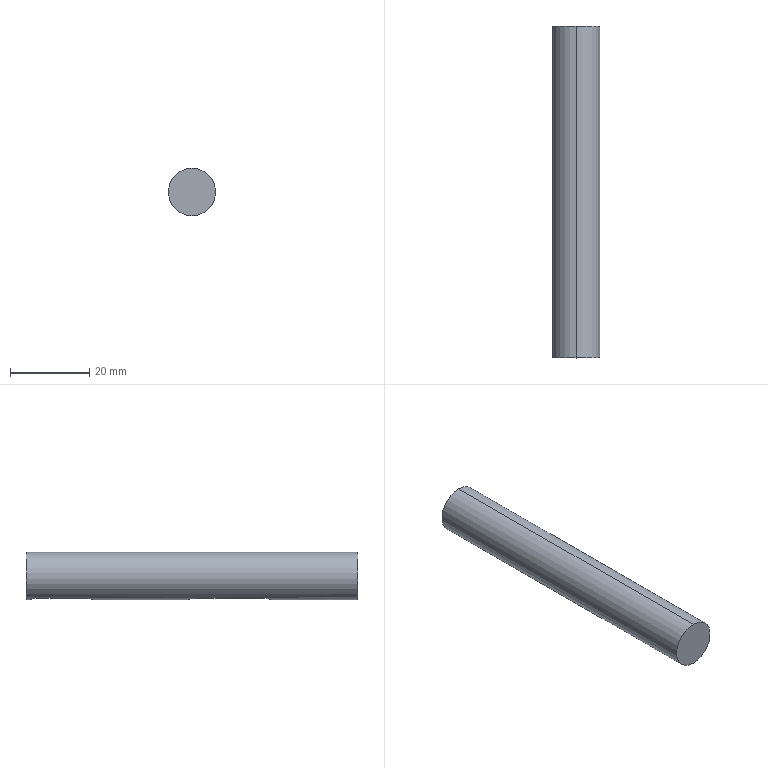Part | 1 solid | 14 faces | box 12 x 84 x 12 mm | volume 9233 mm3 | plane 8 | cylinder 6 | commonest cylinder face diameters 4 x4 12 x2
STEP:
#1=CARTESIAN_POINT('',(0.,84.,6.));
#2=VERTEX_POINT('',#1);
#3=CARTESIAN_POINT('',(0.,84.,-6.));
#4=VERTEX_POINT('',#3);
#5=CARTESIAN_POINT('',(0.,84.,0.));
#6=DIRECTION('',(0.,1.,0.));
#7=DIRECTION('',(0.,0.,1.));
#8=AXIS2_PLACEMENT_3D('',#5,#6,#7);
#9=CIRCLE('',#8,6.);
#10=EDGE_CURVE('',#2,#4,#9,.T.);
#11=ORIENTED_EDGE('',*,*,#10,.F.);
#12=CARTESIAN_POINT('',(0.,0.,6.));
#13=VERTEX_POINT('',#12);
#14=CARTESIAN_POINT('',(0.,84.,6.));
#15=DIRECTION('',(0.,-1.,0.));
#16=VECTOR('',#15,1000.);
#17=LINE('',#14,#16);
#18=EDGE_CURVE('',#2,#13,#17,.T.);
#19=ORIENTED_EDGE('',*,*,#18,.T.);
#20=CARTESIAN_POINT('',(0.,0.,-6.));
#21=VERTEX_POINT('',#20);
#22=CARTESIAN_POINT('',(0.,0.,0.));
#23=DIRECTION('',(0.,1.,0.));
#24=DIRECTION('',(0.,0.,1.));
#25=AXIS2_PLACEMENT_3D('',#22,#23,#24);
#26=CIRCLE('',#25,6.);
#27=EDGE_CURVE('',#13,#21,#26,.T.);
#28=ORIENTED_EDGE('',*,*,#27,.T.);
#29=CARTESIAN_POINT('',(0.,22.,-6.));
#30=VERTEX_POINT('',#29);
#31=CARTESIAN_POINT('',(0.,84.,-6.));
#32=DIRECTION('',(0.,-1.,0.));
#33=VECTOR('',#32,1000.);
#34=LINE('',#31,#33);
#35=EDGE_CURVE('',#30,#21,#34,.T.);
#36=ORIENTED_EDGE('',*,*,#35,.F.);
#37=CARTESIAN_POINT('',(2.,24.,-5.657));
#38=VERTEX_POINT('',#37);
#39=CARTESIAN_POINT('',(0.,22.,-6.));
#40=CARTESIAN_POINT('',(0.1314,22.,-6.));
#41=CARTESIAN_POINT('',(0.2649,22.013,-5.996));
#42=CARTESIAN_POINT('',(0.5219,22.065,-5.979));
#43=CARTESIAN_POINT('',(0.647,22.103,-5.966));
#44=CARTESIAN_POINT('',(0.8902,22.204,-5.935));
#45=CARTESIAN_POINT('',(1.006,22.266,-5.916));
#46=CARTESIAN_POINT('',(1.221,22.411,-5.875));
#47=CARTESIAN_POINT('',(1.323,22.494,-5.853));
#48=CARTESIAN_POINT('',(1.507,22.678,-5.809));
#49=CARTESIAN_POINT('',(1.589,22.778,-5.786));
#50=CARTESIAN_POINT('',(1.733,22.994,-5.745));
#51=CARTESIAN_POINT('',(1.796,23.111,-5.725));
#52=CARTESIAN_POINT('',(1.946,23.471,-5.677));
#53=CARTESIAN_POINT('',(2.,23.734,-5.657));
#54=CARTESIAN_POINT('',(2.,24.,-5.657));
#55=B_SPLINE_CURVE_WITH_KNOTS('',3,(#39,#40,#41,#42,#43,#44,#45,#46,#47,#48,#49,#50,#51,#52,#53,#54),.UNSPECIFIED.,.F.,.F.,(4,2,2,2,2,2,2,4),(0.00315,0.003543,0.003936,0.00433,0.004723,0.005116,0.005509,0.006296),.UNSPECIFIED.);
#56=EDGE_CURVE('',#30,#38,#55,.T.);
#57=ORIENTED_EDGE('',*,*,#56,.T.);
#58=CARTESIAN_POINT('',(2.,41.,-5.657));
#59=VERTEX_POINT('',#58);
#60=CARTESIAN_POINT('',(2.,84.,-5.657));
#61=DIRECTION('',(0.,1.,0.));
#62=VECTOR('',#61,1000.);
#63=LINE('',#60,#62);
#64=EDGE_CURVE('',#38,#59,#63,.T.);
#65=ORIENTED_EDGE('',*,*,#64,.T.);
#66=CARTESIAN_POINT('',(0.,43.,-6.));
#67=VERTEX_POINT('',#66);
#68=CARTESIAN_POINT('',(2.,41.,-5.657));
#69=CARTESIAN_POINT('',(2.,41.132,-5.657));
#70=CARTESIAN_POINT('',(1.987,41.262,-5.661));
#71=CARTESIAN_POINT('',(1.935,41.521,-5.679));
#72=CARTESIAN_POINT('',(1.897,41.648,-5.693));
#73=CARTESIAN_POINT('',(1.746,42.009,-5.741));
#74=CARTESIAN_POINT('',(1.598,42.231,-5.786));
#75=CARTESIAN_POINT('',(1.323,42.506,-5.853));
#76=CARTESIAN_POINT('',(1.221,42.59,-5.876));
#77=CARTESIAN_POINT('',(1.005,42.734,-5.916));
#78=CARTESIAN_POINT('',(0.8903,42.796,-5.935));
#79=CARTESIAN_POINT('',(0.6484,42.896,-5.966));
#80=CARTESIAN_POINT('',(0.5209,42.935,-5.979));
#81=CARTESIAN_POINT('',(0.264,42.987,-5.996));
#82=CARTESIAN_POINT('',(0.1331,43.,-6.));
#83=CARTESIAN_POINT('',(0.,43.,-6.));
#84=B_SPLINE_CURVE_WITH_KNOTS('',3,(#68,#69,#70,#71,#72,#73,#74,#75,#76,#77,#78,#79,#80,#81,#82,#83),.UNSPECIFIED.,.F.,.F.,(4,2,2,2,2,2,2,4),(0.009446,0.00984,0.01023,0.01102,0.01141,0.01181,0.0122,0.0126),.UNSPECIFIED.);
#85=EDGE_CURVE('',#59,#67,#84,.T.);
#86=ORIENTED_EDGE('',*,*,#85,.T.);
#87=CARTESIAN_POINT('',(0.,67.,-6.));
#88=VERTEX_POINT('',#87);
#89=CARTESIAN_POINT('',(0.,84.,-6.));
#90=DIRECTION('',(0.,-1.,0.));
#91=VECTOR('',#90,1000.);
#92=LINE('',#89,#91);
#93=EDGE_CURVE('',#88,#67,#92,.T.);
#94=ORIENTED_EDGE('',*,*,#93,.F.);
#95=CARTESIAN_POINT('',(2.,69.,-5.657));
#96=VERTEX_POINT('',#95);
#97=CARTESIAN_POINT('',(0.,67.,-6.));
#98=CARTESIAN_POINT('',(0.2623,67.,-6.));
#99=CARTESIAN_POINT('',(0.5271,67.053,-5.982));
#100=CARTESIAN_POINT('',(0.889,67.204,-5.935));
#101=CARTESIAN_POINT('',(1.006,67.267,-5.916));
#102=CARTESIAN_POINT('',(1.222,67.411,-5.875));
#103=CARTESIAN_POINT('',(1.322,67.494,-5.853));
#104=CARTESIAN_POINT('',(1.599,67.771,-5.786));
#105=CARTESIAN_POINT('',(1.745,67.989,-5.741));
#106=CARTESIAN_POINT('',(1.897,68.353,-5.692));
#107=CARTESIAN_POINT('',(1.935,68.478,-5.679));
#108=CARTESIAN_POINT('',(1.987,68.735,-5.662));
#109=CARTESIAN_POINT('',(2.,68.868,-5.657));
#110=CARTESIAN_POINT('',(2.,69.,-5.657));
#111=B_SPLINE_CURVE_WITH_KNOTS('',3,(#97,#98,#99,#100,#101,#102,#103,#104,#105,#106,#107,#108,#109,#110),.UNSPECIFIED.,.F.,.F.,(4,2,2,2,2,2,4),(0.006298,0.007085,0.007479,0.007872,0.008659,0.009053,0.009446),.UNSPECIFIED.);
#112=EDGE_CURVE('',#88,#96,#111,.T.);
#113=ORIENTED_EDGE('',*,*,#112,.T.);
#114=CARTESIAN_POINT('',(2.,81.,-5.657));
#115=VERTEX_POINT('',#114);
#116=CARTESIAN_POINT('',(2.,84.,-5.657));
#117=DIRECTION('',(0.,1.,0.));
#118=VECTOR('',#117,1000.);
#119=LINE('',#116,#118);
#120=EDGE_CURVE('',#96,#115,#119,.T.);
#121=ORIENTED_EDGE('',*,*,#120,.T.);
#122=CARTESIAN_POINT('',(0.,83.,-6.));
#123=VERTEX_POINT('',#122);
#124=CARTESIAN_POINT('',(2.,81.,-5.657));
#125=CARTESIAN_POINT('',(2.,81.132,-5.657));
#126=CARTESIAN_POINT('',(1.987,81.262,-5.661));
#127=CARTESIAN_POINT('',(1.935,81.521,-5.679));
#128=CARTESIAN_POINT('',(1.897,81.648,-5.693));
#129=CARTESIAN_POINT('',(1.746,82.009,-5.741));
#130=CARTESIAN_POINT('',(1.598,82.231,-5.786));
#131=CARTESIAN_POINT('',(1.323,82.506,-5.853));
#132=CARTESIAN_POINT('',(1.221,82.59,-5.876));
#133=CARTESIAN_POINT('',(1.005,82.734,-5.916));
#134=CARTESIAN_POINT('',(0.8903,82.796,-5.935));
#135=CARTESIAN_POINT('',(0.6484,82.896,-5.966));
#136=CARTESIAN_POINT('',(0.5209,82.935,-5.979));
#137=CARTESIAN_POINT('',(0.264,82.987,-5.996));
#138=CARTESIAN_POINT('',(0.1331,83.,-6.));
#139=CARTESIAN_POINT('',(0.,83.,-6.));
#140=B_SPLINE_CURVE_WITH_KNOTS('',3,(#124,#125,#126,#127,#128,#129,#130,#131,#132,#133,#134,#135,#136,#137,#138,#139),.UNSPECIFIED.,.F.,.F.,(4,2,2,2,2,2,2,4),(0.009446,0.00984,0.01023,0.01102,0.01141,0.01181,0.0122,0.0126),.UNSPECIFIED.);
#141=EDGE_CURVE('',#115,#123,#140,.T.);
#142=ORIENTED_EDGE('',*,*,#141,.T.);
#143=CARTESIAN_POINT('',(0.,84.,-6.));
#144=DIRECTION('',(0.,-1.,0.));
#145=VECTOR('',#144,1000.);
#146=LINE('',#143,#145);
#147=EDGE_CURVE('',#4,#123,#146,.T.);
#148=ORIENTED_EDGE('',*,*,#147,.F.);
#149=EDGE_LOOP('',(#11,#19,#28,#36,#57,#65,#86,#94,#113,#121,#142,#148));
#150=FACE_OUTER_BOUND('',#149,.T.);
#151=CARTESIAN_POINT('',(0.,84.,0.));
#152=DIRECTION('',(0.,-1.,0.));
#153=DIRECTION('',(0.,0.,-1.));
#154=AXIS2_PLACEMENT_3D('',#151,#152,#153);
#155=CYLINDRICAL_SURFACE('',#154,6.);
#156=ADVANCED_FACE('',(#150),#155,.T.);
#157=ORIENTED_EDGE('',*,*,#18,.F.);
#158=CARTESIAN_POINT('',(0.,84.,0.));
#159=DIRECTION('',(0.,1.,0.));
#160=DIRECTION('',(0.,0.,1.));
#161=AXIS2_PLACEMENT_3D('',#158,#159,#160);
#162=CIRCLE('',#161,6.);
#163=EDGE_CURVE('',#4,#2,#162,.T.);
#164=ORIENTED_EDGE('',*,*,#163,.F.);
#165=ORIENTED_EDGE('',*,*,#147,.T.);
#166=CARTESIAN_POINT('',(-2.,81.,-5.657));
#167=VERTEX_POINT('',#166);
#168=CARTESIAN_POINT('',(0.,83.,-6.));
#169=CARTESIAN_POINT('',(-0.1332,83.,-6.));
#170=CARTESIAN_POINT('',(-0.264,82.987,-5.996));
#171=CARTESIAN_POINT('',(-0.5211,82.935,-5.979));
#172=CARTESIAN_POINT('',(-0.6487,82.896,-5.966));
#173=CARTESIAN_POINT('',(-0.8906,82.796,-5.935));
#174=CARTESIAN_POINT('',(-1.005,82.734,-5.916));
#175=CARTESIAN_POINT('',(-1.222,82.589,-5.875));
#176=CARTESIAN_POINT('',(-1.324,82.505,-5.853));
#177=CARTESIAN_POINT('',(-1.598,82.23,-5.786));
#178=CARTESIAN_POINT('',(-1.747,82.008,-5.741));
#179=CARTESIAN_POINT('',(-1.897,81.648,-5.693));
#180=CARTESIAN_POINT('',(-1.936,81.521,-5.679));
#181=CARTESIAN_POINT('',(-1.987,81.262,-5.661));
#182=CARTESIAN_POINT('',(-2.,81.132,-5.657));
#183=CARTESIAN_POINT('',(-2.,81.,-5.657));
#184=B_SPLINE_CURVE_WITH_KNOTS('',3,(#168,#169,#170,#171,#172,#173,#174,#175,#176,#177,#178,#179,#180,#181,#182,#183),.UNSPECIFIED.,.F.,.F.,(4,2,2,2,2,2,2,4),(0.,0.0003938,0.0007875,0.001181,0.001575,0.002363,0.002756,0.00315),.UNSPECIFIED.);
#185=EDGE_CURVE('',#123,#167,#184,.T.);
#186=ORIENTED_EDGE('',*,*,#185,.T.);
#187=CARTESIAN_POINT('',(-2.,69.,-5.657));
#188=VERTEX_POINT('',#187);
#189=CARTESIAN_POINT('',(-2.,84.,-5.657));
#190=DIRECTION('',(0.,-1.,0.));
#191=VECTOR('',#190,1000.);
#192=LINE('',#189,#191);
#193=EDGE_CURVE('',#167,#188,#192,.T.);
#194=ORIENTED_EDGE('',*,*,#193,.T.);
#195=CARTESIAN_POINT('',(-2.,69.,-5.657));
#196=CARTESIAN_POINT('',(-2.,68.869,-5.657));
#197=CARTESIAN_POINT('',(-1.987,68.735,-5.662));
#198=CARTESIAN_POINT('',(-1.935,68.478,-5.679));
#199=CARTESIAN_POINT('',(-1.897,68.353,-5.693));
#200=CARTESIAN_POINT('',(-1.796,68.109,-5.725));
#201=CARTESIAN_POINT('',(-1.734,67.994,-5.745));
#202=CARTESIAN_POINT('',(-1.589,67.779,-5.786));
#203=CARTESIAN_POINT('',(-1.505,67.677,-5.809));
#204=CARTESIAN_POINT('',(-1.321,67.493,-5.853));
#205=CARTESIAN_POINT('',(-1.221,67.411,-5.875));
#206=CARTESIAN_POINT('',(-1.005,67.266,-5.916));
#207=CARTESIAN_POINT('',(-0.8882,67.203,-5.935));
#208=CARTESIAN_POINT('',(-0.6474,67.103,-5.966));
#209=CARTESIAN_POINT('',(-0.5226,67.065,-5.979));
#210=CARTESIAN_POINT('',(-0.2637,67.013,-5.996));
#211=CARTESIAN_POINT('',(-0.1311,67.,-6.));
#212=CARTESIAN_POINT('',(0.,67.,-6.));
#213=B_SPLINE_CURVE_WITH_KNOTS('',3,(#195,#196,#197,#198,#199,#200,#201,#202,#203,#204,#205,#206,#207,#208,#209,#210,#211,#212),.UNSPECIFIED.,.F.,.F.,(4,2,2,2,2,2,2,2,4),(0.00315,0.003544,0.003937,0.004331,0.004724,0.005118,0.005511,0.005905,0.006298),.UNSPECIFIED.);
#214=EDGE_CURVE('',#188,#88,#213,.T.);
#215=ORIENTED_EDGE('',*,*,#214,.T.);
#216=ORIENTED_EDGE('',*,*,#93,.T.);
#217=CARTESIAN_POINT('',(-2.,41.,-5.657));
#218=VERTEX_POINT('',#217);
#219=CARTESIAN_POINT('',(0.,43.,-6.));
#220=CARTESIAN_POINT('',(-0.1332,43.,-6.));
#221=CARTESIAN_POINT('',(-0.264,42.987,-5.996));
#222=CARTESIAN_POINT('',(-0.5211,42.935,-5.979));
#223=CARTESIAN_POINT('',(-0.6487,42.896,-5.966));
#224=CARTESIAN_POINT('',(-0.8906,42.796,-5.935));
#225=CARTESIAN_POINT('',(-1.005,42.734,-5.916));
#226=CARTESIAN_POINT('',(-1.222,42.589,-5.875));
#227=CARTESIAN_POINT('',(-1.324,42.505,-5.853));
#228=CARTESIAN_POINT('',(-1.598,42.23,-5.786));
#229=CARTESIAN_POINT('',(-1.747,42.008,-5.741));
#230=CARTESIAN_POINT('',(-1.897,41.648,-5.693));
#231=CARTESIAN_POINT('',(-1.936,41.521,-5.679));
#232=CARTESIAN_POINT('',(-1.987,41.262,-5.661));
#233=CARTESIAN_POINT('',(-2.,41.132,-5.657));
#234=CARTESIAN_POINT('',(-2.,41.,-5.657));
#235=B_SPLINE_CURVE_WITH_KNOTS('',3,(#219,#220,#221,#222,#223,#224,#225,#226,#227,#228,#229,#230,#231,#232,#233,#234),.UNSPECIFIED.,.F.,.F.,(4,2,2,2,2,2,2,4),(0.,0.0003938,0.0007875,0.001181,0.001575,0.002363,0.002756,0.00315),.UNSPECIFIED.);
#236=EDGE_CURVE('',#67,#218,#235,.T.);
#237=ORIENTED_EDGE('',*,*,#236,.T.);
#238=CARTESIAN_POINT('',(-2.,24.,-5.657));
#239=VERTEX_POINT('',#238);
#240=CARTESIAN_POINT('',(-2.,84.,-5.657));
#241=DIRECTION('',(0.,-1.,0.));
#242=VECTOR('',#241,1000.);
#243=LINE('',#240,#242);
#244=EDGE_CURVE('',#218,#239,#243,.T.);
#245=ORIENTED_EDGE('',*,*,#244,.T.);
#246=CARTESIAN_POINT('',(-2.,24.,-5.657));
#247=CARTESIAN_POINT('',(-2.,23.867,-5.657));
#248=CARTESIAN_POINT('',(-1.987,23.736,-5.662));
#249=CARTESIAN_POINT('',(-1.935,23.479,-5.679));
#250=CARTESIAN_POINT('',(-1.896,23.351,-5.693));
#251=CARTESIAN_POINT('',(-1.796,23.11,-5.725));
#252=CARTESIAN_POINT('',(-1.734,22.995,-5.744));
#253=CARTESIAN_POINT('',(-1.589,22.779,-5.786));
#254=CARTESIAN_POINT('',(-1.505,22.677,-5.809));
#255=CARTESIAN_POINT('',(-1.23,22.402,-5.876));
#256=CARTESIAN_POINT('',(-1.009,22.253,-5.92));
#257=CARTESIAN_POINT('',(-0.648,22.103,-5.966));
#258=CARTESIAN_POINT('',(-0.5209,22.065,-5.979));
#259=CARTESIAN_POINT('',(-0.2621,22.013,-5.996));
#260=CARTESIAN_POINT('',(-0.1316,22.,-6.));
#261=CARTESIAN_POINT('',(0.,22.,-6.));
#262=B_SPLINE_CURVE_WITH_KNOTS('',3,(#246,#247,#248,#249,#250,#251,#252,#253,#254,#255,#256,#257,#258,#259,#260,#261),.UNSPECIFIED.,.F.,.F.,(4,2,2,2,2,2,2,4),(0.,0.0003937,0.0007875,0.001181,0.001575,0.002362,0.002756,0.00315),.UNSPECIFIED.);
#263=EDGE_CURVE('',#239,#30,#262,.T.);
#264=ORIENTED_EDGE('',*,*,#263,.T.);
#265=ORIENTED_EDGE('',*,*,#35,.T.);
#266=CARTESIAN_POINT('',(0.,0.,0.));
#267=DIRECTION('',(0.,1.,0.));
#268=DIRECTION('',(0.,0.,1.));
#269=AXIS2_PLACEMENT_3D('',#266,#267,#268);
#270=CIRCLE('',#269,6.);
#271=EDGE_CURVE('',#21,#13,#270,.T.);
#272=ORIENTED_EDGE('',*,*,#271,.T.);
#273=EDGE_LOOP('',(#157,#164,#165,#186,#194,#215,#216,#237,#245,#264,#265,#272));
#274=FACE_OUTER_BOUND('',#273,.T.);
#275=CARTESIAN_POINT('',(0.,84.,0.));
#276=DIRECTION('',(0.,-1.,0.));
#277=DIRECTION('',(0.,0.,-1.));
#278=AXIS2_PLACEMENT_3D('',#275,#276,#277);
#279=CYLINDRICAL_SURFACE('',#278,6.);
#280=ADVANCED_FACE('',(#274),#279,.T.);
#281=ORIENTED_EDGE('',*,*,#163,.T.);
#282=ORIENTED_EDGE('',*,*,#10,.T.);
#283=EDGE_LOOP('',(#281,#282));
#284=FACE_OUTER_BOUND('',#283,.T.);
#285=CARTESIAN_POINT('',(0.,84.,0.));
#286=DIRECTION('',(0.,1.,0.));
#287=DIRECTION('',(0.,0.,1.));
#288=AXIS2_PLACEMENT_3D('',#285,#286,#287);
#289=PLANE('',#288);
#290=ADVANCED_FACE('',(#284),#289,.T.);
#291=ORIENTED_EDGE('',*,*,#271,.F.);
#292=ORIENTED_EDGE('',*,*,#27,.F.);
#293=EDGE_LOOP('',(#291,#292));
#294=FACE_OUTER_BOUND('',#293,.T.);
#295=CARTESIAN_POINT('',(0.,0.,0.));
#296=DIRECTION('',(0.,1.,0.));
#297=DIRECTION('',(0.,0.,1.));
#298=AXIS2_PLACEMENT_3D('',#295,#296,#297);
#299=PLANE('',#298);
#300=ADVANCED_FACE('',(#294),#299,.F.);
#301=CARTESIAN_POINT('',(-2.,24.,-4.));
#302=VERTEX_POINT('',#301);
#303=CARTESIAN_POINT('',(-2.,24.,-19.));
#304=DIRECTION('',(0.,0.,1.));
#305=VECTOR('',#304,1000.);
#306=LINE('',#303,#305);
#307=EDGE_CURVE('',#239,#302,#306,.T.);
#308=ORIENTED_EDGE('',*,*,#307,.T.);
#309=CARTESIAN_POINT('',(2.,24.,-4.));
#310=VERTEX_POINT('',#309);
#311=CARTESIAN_POINT('',(0.,24.,-4.));
#312=DIRECTION('',(0.,0.,1.));
#313=DIRECTION('',(1.,0.,0.));
#314=AXIS2_PLACEMENT_3D('',#311,#312,#313);
#315=CIRCLE('',#314,2.);
#316=EDGE_CURVE('',#302,#310,#315,.T.);
#317=ORIENTED_EDGE('',*,*,#316,.T.);
#318=CARTESIAN_POINT('',(2.,24.,-19.));
#319=DIRECTION('',(0.,0.,1.));
#320=VECTOR('',#319,1000.);
#321=LINE('',#318,#320);
#322=EDGE_CURVE('',#38,#310,#321,.T.);
#323=ORIENTED_EDGE('',*,*,#322,.F.);
#324=ORIENTED_EDGE('',*,*,#56,.F.);
#325=ORIENTED_EDGE('',*,*,#263,.F.);
#326=EDGE_LOOP('',(#308,#317,#323,#324,#325));
#327=FACE_OUTER_BOUND('',#326,.T.);
#328=CARTESIAN_POINT('',(0.,24.,-19.));
#329=DIRECTION('',(0.,0.,1.));
#330=DIRECTION('',(1.,0.,0.));
#331=AXIS2_PLACEMENT_3D('',#328,#329,#330);
#332=CYLINDRICAL_SURFACE('',#331,2.);
#333=ADVANCED_FACE('',(#327),#332,.F.);
#334=CARTESIAN_POINT('',(-2.,41.,-4.));
#335=VERTEX_POINT('',#334);
#336=CARTESIAN_POINT('',(-2.,41.,-19.));
#337=DIRECTION('',(0.,0.,1.));
#338=VECTOR('',#337,1000.);
#339=LINE('',#336,#338);
#340=EDGE_CURVE('',#218,#335,#339,.T.);
#341=ORIENTED_EDGE('',*,*,#340,.T.);
#342=CARTESIAN_POINT('',(-2.,24.,-4.));
#343=DIRECTION('',(0.,-1.,0.));
#344=VECTOR('',#343,1000.);
#345=LINE('',#342,#344);
#346=EDGE_CURVE('',#335,#302,#345,.T.);
#347=ORIENTED_EDGE('',*,*,#346,.T.);
#348=ORIENTED_EDGE('',*,*,#307,.F.);
#349=ORIENTED_EDGE('',*,*,#244,.F.);
#350=EDGE_LOOP('',(#341,#347,#348,#349));
#351=FACE_OUTER_BOUND('',#350,.T.);
#352=CARTESIAN_POINT('',(-2.,24.,-19.));
#353=DIRECTION('',(-1.,0.,0.));
#354=DIRECTION('',(0.,0.,1.));
#355=AXIS2_PLACEMENT_3D('',#352,#353,#354);
#356=PLANE('',#355);
#357=ADVANCED_FACE('',(#351),#356,.F.);
#358=CARTESIAN_POINT('',(2.,41.,-4.));
#359=VERTEX_POINT('',#358);
#360=CARTESIAN_POINT('',(2.,41.,-19.));
#361=DIRECTION('',(0.,0.,1.));
#362=VECTOR('',#361,1000.);
#363=LINE('',#360,#362);
#364=EDGE_CURVE('',#59,#359,#363,.T.);
#365=ORIENTED_EDGE('',*,*,#364,.T.);
#366=CARTESIAN_POINT('',(0.,41.,-4.));
#367=DIRECTION('',(0.,0.,1.));
#368=DIRECTION('',(1.,0.,0.));
#369=AXIS2_PLACEMENT_3D('',#366,#367,#368);
#370=CIRCLE('',#369,2.);
#371=EDGE_CURVE('',#359,#335,#370,.T.);
#372=ORIENTED_EDGE('',*,*,#371,.T.);
#373=ORIENTED_EDGE('',*,*,#340,.F.);
#374=ORIENTED_EDGE('',*,*,#236,.F.);
#375=ORIENTED_EDGE('',*,*,#85,.F.);
#376=EDGE_LOOP('',(#365,#372,#373,#374,#375));
#377=FACE_OUTER_BOUND('',#376,.T.);
#378=CARTESIAN_POINT('',(0.,41.,-19.));
#379=DIRECTION('',(0.,0.,1.));
#380=DIRECTION('',(1.,0.,0.));
#381=AXIS2_PLACEMENT_3D('',#378,#379,#380);
#382=CYLINDRICAL_SURFACE('',#381,2.);
#383=ADVANCED_FACE('',(#377),#382,.F.);
#384=ORIENTED_EDGE('',*,*,#322,.T.);
#385=CARTESIAN_POINT('',(2.,24.,-4.));
#386=DIRECTION('',(0.,1.,0.));
#387=VECTOR('',#386,1000.);
#388=LINE('',#385,#387);
#389=EDGE_CURVE('',#310,#359,#388,.T.);
#390=ORIENTED_EDGE('',*,*,#389,.T.);
#391=ORIENTED_EDGE('',*,*,#364,.F.);
#392=ORIENTED_EDGE('',*,*,#64,.F.);
#393=EDGE_LOOP('',(#384,#390,#391,#392));
#394=FACE_OUTER_BOUND('',#393,.T.);
#395=CARTESIAN_POINT('',(2.,24.,-19.));
#396=DIRECTION('',(1.,0.,0.));
#397=DIRECTION('',(0.,0.,-1.));
#398=AXIS2_PLACEMENT_3D('',#395,#396,#397);
#399=PLANE('',#398);
#400=ADVANCED_FACE('',(#394),#399,.F.);
#401=ORIENTED_EDGE('',*,*,#316,.F.);
#402=ORIENTED_EDGE('',*,*,#346,.F.);
#403=ORIENTED_EDGE('',*,*,#371,.F.);
#404=ORIENTED_EDGE('',*,*,#389,.F.);
#405=EDGE_LOOP('',(#401,#402,#403,#404));
#406=FACE_OUTER_BOUND('',#405,.T.);
#407=CARTESIAN_POINT('',(0.,24.,-4.));
#408=DIRECTION('',(0.,0.,1.));
#409=DIRECTION('',(1.,0.,0.));
#410=AXIS2_PLACEMENT_3D('',#407,#408,#409);
#411=PLANE('',#410);
#412=ADVANCED_FACE('',(#406),#411,.F.);
#413=CARTESIAN_POINT('',(2.,81.,-4.));
#414=VERTEX_POINT('',#413);
#415=CARTESIAN_POINT('',(2.,81.,-19.));
#416=DIRECTION('',(0.,0.,1.));
#417=VECTOR('',#416,1000.);
#418=LINE('',#415,#417);
#419=EDGE_CURVE('',#115,#414,#418,.T.);
#420=ORIENTED_EDGE('',*,*,#419,.T.);
#421=CARTESIAN_POINT('',(-2.,81.,-4.));
#422=VERTEX_POINT('',#421);
#423=CARTESIAN_POINT('',(0.,81.,-4.));
#424=DIRECTION('',(0.,0.,1.));
#425=DIRECTION('',(1.,0.,0.));
#426=AXIS2_PLACEMENT_3D('',#423,#424,#425);
#427=CIRCLE('',#426,2.);
#428=EDGE_CURVE('',#414,#422,#427,.T.);
#429=ORIENTED_EDGE('',*,*,#428,.T.);
#430=CARTESIAN_POINT('',(-2.,81.,-19.));
#431=DIRECTION('',(0.,0.,1.));
#432=VECTOR('',#431,1000.);
#433=LINE('',#430,#432);
#434=EDGE_CURVE('',#167,#422,#433,.T.);
#435=ORIENTED_EDGE('',*,*,#434,.F.);
#436=ORIENTED_EDGE('',*,*,#185,.F.);
#437=ORIENTED_EDGE('',*,*,#141,.F.);
#438=EDGE_LOOP('',(#420,#429,#435,#436,#437));
#439=FACE_OUTER_BOUND('',#438,.T.);
#440=CARTESIAN_POINT('',(0.,81.,-19.));
#441=DIRECTION('',(0.,0.,1.));
#442=DIRECTION('',(1.,0.,0.));
#443=AXIS2_PLACEMENT_3D('',#440,#441,#442);
#444=CYLINDRICAL_SURFACE('',#443,2.);
#445=ADVANCED_FACE('',(#439),#444,.F.);
#446=CARTESIAN_POINT('',(2.,69.,-4.));
#447=VERTEX_POINT('',#446);
#448=CARTESIAN_POINT('',(2.,69.,-19.));
#449=DIRECTION('',(0.,0.,1.));
#450=VECTOR('',#449,1000.);
#451=LINE('',#448,#450);
#452=EDGE_CURVE('',#96,#447,#451,.T.);
#453=ORIENTED_EDGE('',*,*,#452,.T.);
#454=CARTESIAN_POINT('',(2.,81.,-4.));
#455=DIRECTION('',(0.,1.,0.));
#456=VECTOR('',#455,1000.);
#457=LINE('',#454,#456);
#458=EDGE_CURVE('',#447,#414,#457,.T.);
#459=ORIENTED_EDGE('',*,*,#458,.T.);
#460=ORIENTED_EDGE('',*,*,#419,.F.);
#461=ORIENTED_EDGE('',*,*,#120,.F.);
#462=EDGE_LOOP('',(#453,#459,#460,#461));
#463=FACE_OUTER_BOUND('',#462,.T.);
#464=CARTESIAN_POINT('',(2.,81.,-19.));
#465=DIRECTION('',(1.,0.,0.));
#466=DIRECTION('',(0.,1.,0.));
#467=AXIS2_PLACEMENT_3D('',#464,#465,#466);
#468=PLANE('',#467);
#469=ADVANCED_FACE('',(#463),#468,.F.);
#470=CARTESIAN_POINT('',(-2.,69.,-4.));
#471=VERTEX_POINT('',#470);
#472=CARTESIAN_POINT('',(-2.,69.,-19.));
#473=DIRECTION('',(0.,0.,1.));
#474=VECTOR('',#473,1000.);
#475=LINE('',#472,#474);
#476=EDGE_CURVE('',#188,#471,#475,.T.);
#477=ORIENTED_EDGE('',*,*,#476,.T.);
#478=CARTESIAN_POINT('',(0.,69.,-4.));
#479=DIRECTION('',(0.,0.,1.));
#480=DIRECTION('',(1.,0.,0.));
#481=AXIS2_PLACEMENT_3D('',#478,#479,#480);
#482=CIRCLE('',#481,2.);
#483=EDGE_CURVE('',#471,#447,#482,.T.);
#484=ORIENTED_EDGE('',*,*,#483,.T.);
#485=ORIENTED_EDGE('',*,*,#452,.F.);
#486=ORIENTED_EDGE('',*,*,#112,.F.);
#487=ORIENTED_EDGE('',*,*,#214,.F.);
#488=EDGE_LOOP('',(#477,#484,#485,#486,#487));
#489=FACE_OUTER_BOUND('',#488,.T.);
#490=CARTESIAN_POINT('',(0.,69.,-19.));
#491=DIRECTION('',(0.,0.,1.));
#492=DIRECTION('',(1.,0.,0.));
#493=AXIS2_PLACEMENT_3D('',#490,#491,#492);
#494=CYLINDRICAL_SURFACE('',#493,2.);
#495=ADVANCED_FACE('',(#489),#494,.F.);
#496=ORIENTED_EDGE('',*,*,#434,.T.);
#497=CARTESIAN_POINT('',(-2.,81.,-4.));
#498=DIRECTION('',(0.,-1.,0.));
#499=VECTOR('',#498,1000.);
#500=LINE('',#497,#499);
#501=EDGE_CURVE('',#422,#471,#500,.T.);
#502=ORIENTED_EDGE('',*,*,#501,.T.);
#503=ORIENTED_EDGE('',*,*,#476,.F.);
#504=ORIENTED_EDGE('',*,*,#193,.F.);
#505=EDGE_LOOP('',(#496,#502,#503,#504));
#506=FACE_OUTER_BOUND('',#505,.T.);
#507=CARTESIAN_POINT('',(-2.,81.,-19.));
#508=DIRECTION('',(-1.,0.,0.));
#509=DIRECTION('',(0.,-1.,0.));
#510=AXIS2_PLACEMENT_3D('',#507,#508,#509);
#511=PLANE('',#510);
#512=ADVANCED_FACE('',(#506),#511,.F.);
#513=ORIENTED_EDGE('',*,*,#428,.F.);
#514=ORIENTED_EDGE('',*,*,#458,.F.);
#515=ORIENTED_EDGE('',*,*,#483,.F.);
#516=ORIENTED_EDGE('',*,*,#501,.F.);
#517=EDGE_LOOP('',(#513,#514,#515,#516));
#518=FACE_OUTER_BOUND('',#517,.T.);
#519=CARTESIAN_POINT('',(0.,81.,-4.));
#520=DIRECTION('',(0.,0.,1.));
#521=DIRECTION('',(1.,0.,0.));
#522=AXIS2_PLACEMENT_3D('',#519,#520,#521);
#523=PLANE('',#522);
#524=ADVANCED_FACE('',(#518),#523,.F.);
#525=CLOSED_SHELL('',(#156,#280,#290,#300,#333,#357,#383,#400,#412,#445,#469,#495,#512,#524));
#526=MANIFOLD_SOLID_BREP('',#525);
#527=CARTESIAN_POINT('',(0.,0.,0.));
#528=DIRECTION('',(0.,0.,1.));
#529=DIRECTION('',(1.,0.,0.));
#530=AXIS2_PLACEMENT_3D('',#527,#528,#529);
#531=(LENGTH_UNIT()NAMED_UNIT(*)SI_UNIT(.MILLI.,.METRE.));
#532=UNCERTAINTY_MEASURE_WITH_UNIT(LENGTH_MEASURE(0.00001),#531,'','');
#533=(NAMED_UNIT(*)PLANE_ANGLE_UNIT()SI_UNIT($,.RADIAN.));
#534=(NAMED_UNIT(*)SI_UNIT($,.STERADIAN.)SOLID_ANGLE_UNIT());
#535=(GEOMETRIC_REPRESENTATION_CONTEXT(3)GLOBAL_UNCERTAINTY_ASSIGNED_CONTEXT((#532))GLOBAL_UNIT_ASSIGNED_CONTEXT((#531,#533,#534))REPRESENTATION_CONTEXT('',''));
#536=ADVANCED_BREP_SHAPE_REPRESENTATION('',(#526,#530),#535);